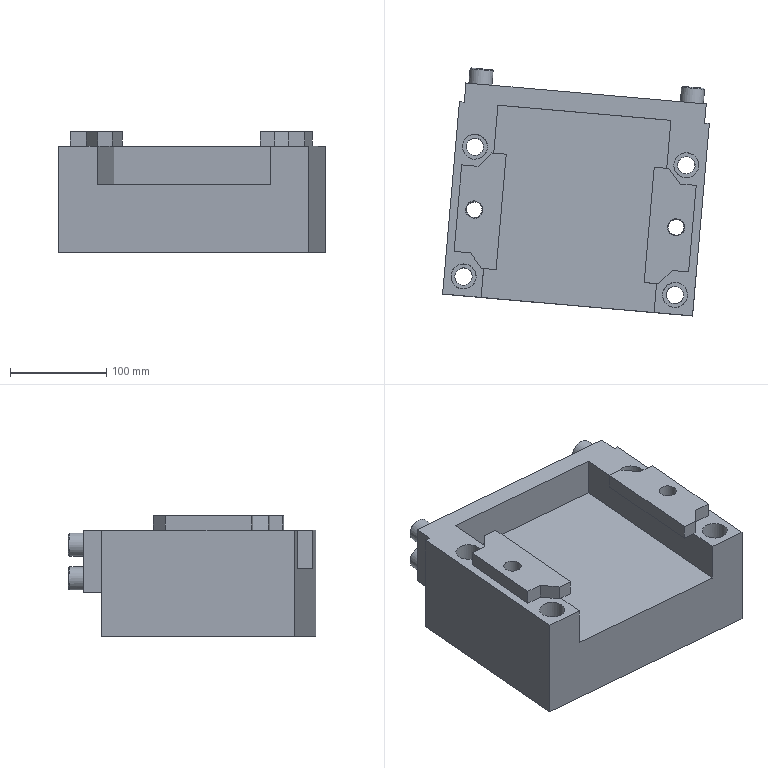Part | NX | features solid 2 | 1 solid | 68 faces | box 276.442 x 256.978 x 125 mm | volume 4551984 mm3 | plane 46 | cylinder 18 | cone 4 | commonest cylinder face diameters 18 x6 24 x4 26 x4 16 x2 17 x2